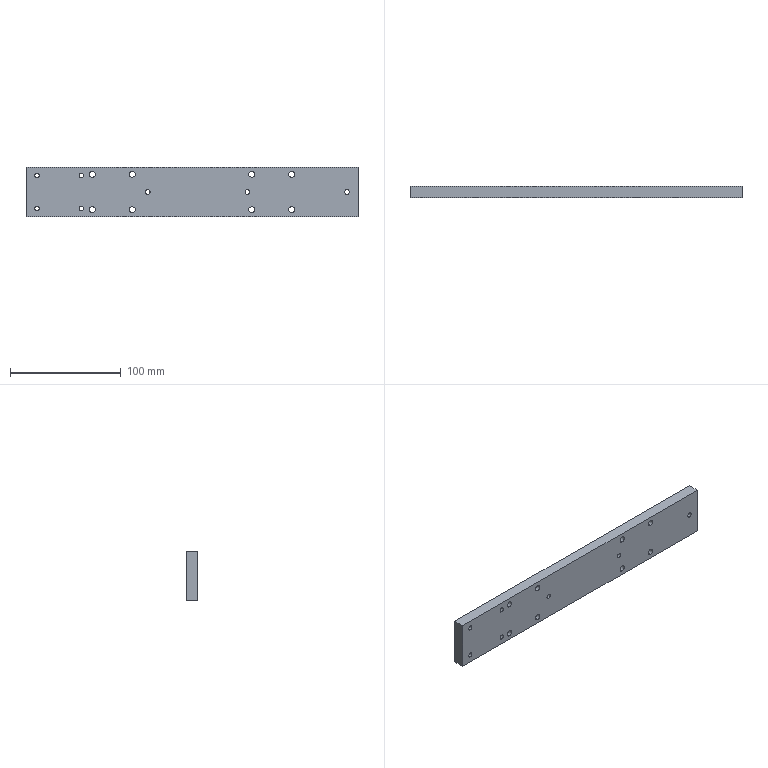Part | STEP file | Dust cover sliding base plate | 1 solid | 60 faces | box 300 x 10 x 45 mm | volume 129631 mm3 | cylinder 46 | plane 14 | commonest cylinder face diameters 5.5 x16 10 x16 4.2 x14